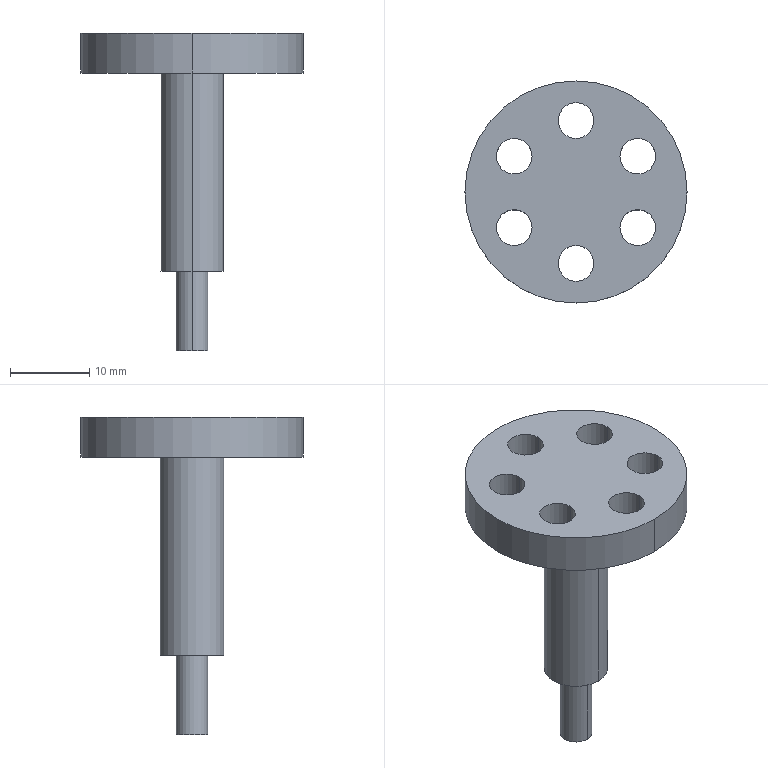Part | STEP file | 04-18 Gear support column | 1 solid | 22 faces | box 28 x 28 x 40 mm | volume 3984 mm3 | cylinder 18 | plane 4 | commonest cylinder face diameters 4.5 x12 4 x2 8 x2 28 x2